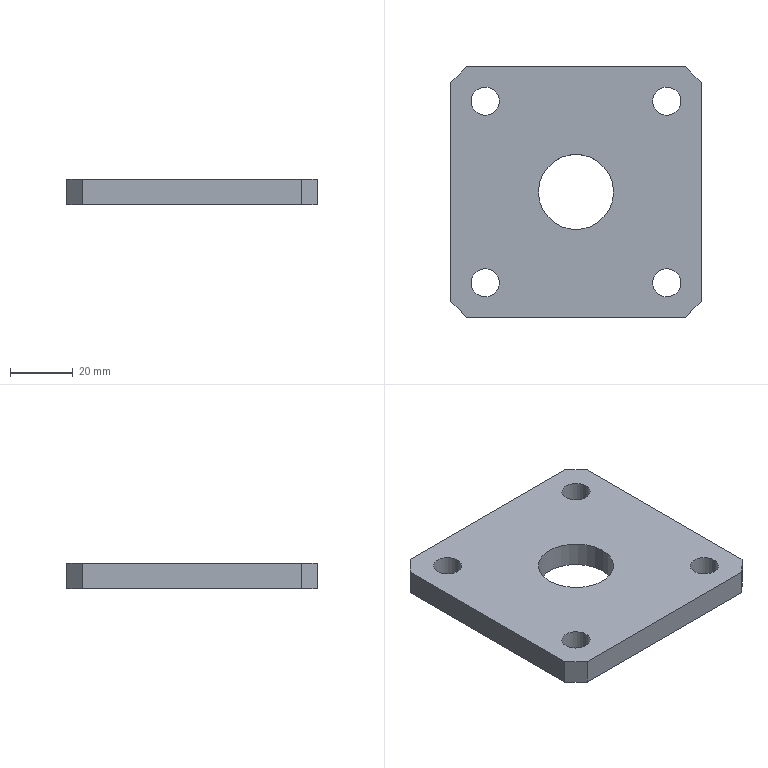Part | SolidWorks | features Chamfer 1, Extrusion 1 | 1 solid | 20 faces | box 80 x 80 x 8 mm | volume 45145 mm3 | cylinder 10 | plane 10 | commonest cylinder face diameters 9 x8 24 x2
STEP:
#1=CARTESIAN_POINT('',(23.386,38.474,8.));
#2=VERTEX_POINT('',#1);
#3=CARTESIAN_POINT('',(32.386,38.474,8.));
#4=VERTEX_POINT('',#3);
#5=CARTESIAN_POINT('',(27.886,38.474,8.));
#6=DIRECTION('',(0.,0.,1.));
#7=DIRECTION('',(1.,0.,0.));
#8=AXIS2_PLACEMENT_3D('',#5,#6,#7);
#9=CIRCLE('',#8,4.5);
#10=EDGE_CURVE('',#2,#4,#9,.T.);
#11=ORIENTED_EDGE('',*,*,#10,.T.);
#12=CARTESIAN_POINT('',(32.386,38.474,0.));
#13=VERTEX_POINT('',#12);
#14=CARTESIAN_POINT('',(32.386,38.474,8.));
#15=DIRECTION('',(0.,0.,-1.));
#16=VECTOR('',#15,1000.);
#17=LINE('',#14,#16);
#18=EDGE_CURVE('',#4,#13,#17,.T.);
#19=ORIENTED_EDGE('',*,*,#18,.T.);
#20=CARTESIAN_POINT('',(23.386,38.474,0.));
#21=VERTEX_POINT('',#20);
#22=CARTESIAN_POINT('',(27.886,38.474,0.));
#23=DIRECTION('',(0.,0.,1.));
#24=DIRECTION('',(1.,0.,0.));
#25=AXIS2_PLACEMENT_3D('',#22,#23,#24);
#26=CIRCLE('',#25,4.5);
#27=EDGE_CURVE('',#21,#13,#26,.T.);
#28=ORIENTED_EDGE('',*,*,#27,.F.);
#29=CARTESIAN_POINT('',(23.386,38.474,8.));
#30=DIRECTION('',(0.,0.,-1.));
#31=VECTOR('',#30,1000.);
#32=LINE('',#29,#31);
#33=EDGE_CURVE('',#2,#21,#32,.T.);
#34=ORIENTED_EDGE('',*,*,#33,.F.);
#35=EDGE_LOOP('',(#11,#19,#28,#34));
#36=FACE_OUTER_BOUND('',#35,.T.);
#37=CARTESIAN_POINT('',(27.886,38.474,8.));
#38=DIRECTION('',(0.,0.,-1.));
#39=DIRECTION('',(-1.,0.,0.));
#40=AXIS2_PLACEMENT_3D('',#37,#38,#39);
#41=CYLINDRICAL_SURFACE('',#40,4.5);
#42=ADVANCED_FACE('',(#36),#41,.F.);
#43=CARTESIAN_POINT('',(23.386,-19.526,8.));
#44=VERTEX_POINT('',#43);
#45=CARTESIAN_POINT('',(32.386,-19.526,8.));
#46=VERTEX_POINT('',#45);
#47=CARTESIAN_POINT('',(27.886,-19.526,8.));
#48=DIRECTION('',(0.,0.,1.));
#49=DIRECTION('',(1.,0.,0.));
#50=AXIS2_PLACEMENT_3D('',#47,#48,#49);
#51=CIRCLE('',#50,4.5);
#52=EDGE_CURVE('',#44,#46,#51,.T.);
#53=ORIENTED_EDGE('',*,*,#52,.T.);
#54=CARTESIAN_POINT('',(32.386,-19.526,0.));
#55=VERTEX_POINT('',#54);
#56=CARTESIAN_POINT('',(32.386,-19.526,8.));
#57=DIRECTION('',(0.,0.,-1.));
#58=VECTOR('',#57,1000.);
#59=LINE('',#56,#58);
#60=EDGE_CURVE('',#46,#55,#59,.T.);
#61=ORIENTED_EDGE('',*,*,#60,.T.);
#62=CARTESIAN_POINT('',(23.386,-19.526,0.));
#63=VERTEX_POINT('',#62);
#64=CARTESIAN_POINT('',(27.886,-19.526,0.));
#65=DIRECTION('',(0.,0.,1.));
#66=DIRECTION('',(1.,0.,0.));
#67=AXIS2_PLACEMENT_3D('',#64,#65,#66);
#68=CIRCLE('',#67,4.5);
#69=EDGE_CURVE('',#63,#55,#68,.T.);
#70=ORIENTED_EDGE('',*,*,#69,.F.);
#71=CARTESIAN_POINT('',(23.386,-19.526,8.));
#72=DIRECTION('',(0.,0.,-1.));
#73=VECTOR('',#72,1000.);
#74=LINE('',#71,#73);
#75=EDGE_CURVE('',#44,#63,#74,.T.);
#76=ORIENTED_EDGE('',*,*,#75,.F.);
#77=EDGE_LOOP('',(#53,#61,#70,#76));
#78=FACE_OUTER_BOUND('',#77,.T.);
#79=CARTESIAN_POINT('',(27.886,-19.526,8.));
#80=DIRECTION('',(0.,0.,-1.));
#81=DIRECTION('',(-1.,0.,0.));
#82=AXIS2_PLACEMENT_3D('',#79,#80,#81);
#83=CYLINDRICAL_SURFACE('',#82,4.5);
#84=ADVANCED_FACE('',(#78),#83,.F.);
#85=CARTESIAN_POINT('',(-34.614,-19.526,8.));
#86=VERTEX_POINT('',#85);
#87=CARTESIAN_POINT('',(-25.614,-19.526,8.));
#88=VERTEX_POINT('',#87);
#89=CARTESIAN_POINT('',(-30.114,-19.526,8.));
#90=DIRECTION('',(0.,0.,1.));
#91=DIRECTION('',(1.,0.,0.));
#92=AXIS2_PLACEMENT_3D('',#89,#90,#91);
#93=CIRCLE('',#92,4.5);
#94=EDGE_CURVE('',#86,#88,#93,.T.);
#95=ORIENTED_EDGE('',*,*,#94,.T.);
#96=CARTESIAN_POINT('',(-25.614,-19.526,0.));
#97=VERTEX_POINT('',#96);
#98=CARTESIAN_POINT('',(-25.614,-19.526,8.));
#99=DIRECTION('',(0.,0.,-1.));
#100=VECTOR('',#99,1000.);
#101=LINE('',#98,#100);
#102=EDGE_CURVE('',#88,#97,#101,.T.);
#103=ORIENTED_EDGE('',*,*,#102,.T.);
#104=CARTESIAN_POINT('',(-34.614,-19.526,0.));
#105=VERTEX_POINT('',#104);
#106=CARTESIAN_POINT('',(-30.114,-19.526,0.));
#107=DIRECTION('',(0.,0.,1.));
#108=DIRECTION('',(1.,0.,0.));
#109=AXIS2_PLACEMENT_3D('',#106,#107,#108);
#110=CIRCLE('',#109,4.5);
#111=EDGE_CURVE('',#105,#97,#110,.T.);
#112=ORIENTED_EDGE('',*,*,#111,.F.);
#113=CARTESIAN_POINT('',(-34.614,-19.526,8.));
#114=DIRECTION('',(0.,0.,-1.));
#115=VECTOR('',#114,1000.);
#116=LINE('',#113,#115);
#117=EDGE_CURVE('',#86,#105,#116,.T.);
#118=ORIENTED_EDGE('',*,*,#117,.F.);
#119=EDGE_LOOP('',(#95,#103,#112,#118));
#120=FACE_OUTER_BOUND('',#119,.T.);
#121=CARTESIAN_POINT('',(-30.114,-19.526,8.));
#122=DIRECTION('',(0.,0.,-1.));
#123=DIRECTION('',(-1.,0.,0.));
#124=AXIS2_PLACEMENT_3D('',#121,#122,#123);
#125=CYLINDRICAL_SURFACE('',#124,4.5);
#126=ADVANCED_FACE('',(#120),#125,.F.);
#127=CARTESIAN_POINT('',(-34.614,38.474,8.));
#128=VERTEX_POINT('',#127);
#129=CARTESIAN_POINT('',(-25.614,38.474,8.));
#130=VERTEX_POINT('',#129);
#131=CARTESIAN_POINT('',(-30.114,38.474,8.));
#132=DIRECTION('',(0.,0.,1.));
#133=DIRECTION('',(1.,0.,0.));
#134=AXIS2_PLACEMENT_3D('',#131,#132,#133);
#135=CIRCLE('',#134,4.5);
#136=EDGE_CURVE('',#128,#130,#135,.T.);
#137=ORIENTED_EDGE('',*,*,#136,.T.);
#138=CARTESIAN_POINT('',(-25.614,38.474,0.));
#139=VERTEX_POINT('',#138);
#140=CARTESIAN_POINT('',(-25.614,38.474,8.));
#141=DIRECTION('',(0.,0.,-1.));
#142=VECTOR('',#141,1000.);
#143=LINE('',#140,#142);
#144=EDGE_CURVE('',#130,#139,#143,.T.);
#145=ORIENTED_EDGE('',*,*,#144,.T.);
#146=CARTESIAN_POINT('',(-34.614,38.474,0.));
#147=VERTEX_POINT('',#146);
#148=CARTESIAN_POINT('',(-30.114,38.474,0.));
#149=DIRECTION('',(0.,0.,1.));
#150=DIRECTION('',(1.,0.,0.));
#151=AXIS2_PLACEMENT_3D('',#148,#149,#150);
#152=CIRCLE('',#151,4.5);
#153=EDGE_CURVE('',#147,#139,#152,.T.);
#154=ORIENTED_EDGE('',*,*,#153,.F.);
#155=CARTESIAN_POINT('',(-34.614,38.474,8.));
#156=DIRECTION('',(0.,0.,-1.));
#157=VECTOR('',#156,1000.);
#158=LINE('',#155,#157);
#159=EDGE_CURVE('',#128,#147,#158,.T.);
#160=ORIENTED_EDGE('',*,*,#159,.F.);
#161=EDGE_LOOP('',(#137,#145,#154,#160));
#162=FACE_OUTER_BOUND('',#161,.T.);
#163=CARTESIAN_POINT('',(-30.114,38.474,8.));
#164=DIRECTION('',(0.,0.,-1.));
#165=DIRECTION('',(-1.,0.,0.));
#166=AXIS2_PLACEMENT_3D('',#163,#164,#165);
#167=CYLINDRICAL_SURFACE('',#166,4.5);
#168=ADVANCED_FACE('',(#162),#167,.F.);
#169=CARTESIAN_POINT('',(-13.114,9.474,8.));
#170=VERTEX_POINT('',#169);
#171=CARTESIAN_POINT('',(10.886,9.474,8.));
#172=VERTEX_POINT('',#171);
#173=CARTESIAN_POINT('',(-1.114,9.474,8.));
#174=DIRECTION('',(0.,0.,1.));
#175=DIRECTION('',(1.,0.,0.));
#176=AXIS2_PLACEMENT_3D('',#173,#174,#175);
#177=CIRCLE('',#176,12.);
#178=EDGE_CURVE('',#170,#172,#177,.T.);
#179=ORIENTED_EDGE('',*,*,#178,.T.);
#180=CARTESIAN_POINT('',(10.886,9.474,0.));
#181=VERTEX_POINT('',#180);
#182=CARTESIAN_POINT('',(10.886,9.474,8.));
#183=DIRECTION('',(0.,0.,-1.));
#184=VECTOR('',#183,1000.);
#185=LINE('',#182,#184);
#186=EDGE_CURVE('',#172,#181,#185,.T.);
#187=ORIENTED_EDGE('',*,*,#186,.T.);
#188=CARTESIAN_POINT('',(-13.114,9.474,0.));
#189=VERTEX_POINT('',#188);
#190=CARTESIAN_POINT('',(-1.114,9.474,0.));
#191=DIRECTION('',(0.,0.,1.));
#192=DIRECTION('',(1.,0.,0.));
#193=AXIS2_PLACEMENT_3D('',#190,#191,#192);
#194=CIRCLE('',#193,12.);
#195=EDGE_CURVE('',#189,#181,#194,.T.);
#196=ORIENTED_EDGE('',*,*,#195,.F.);
#197=CARTESIAN_POINT('',(-13.114,9.474,8.));
#198=DIRECTION('',(0.,0.,-1.));
#199=VECTOR('',#198,1000.);
#200=LINE('',#197,#199);
#201=EDGE_CURVE('',#170,#189,#200,.T.);
#202=ORIENTED_EDGE('',*,*,#201,.F.);
#203=EDGE_LOOP('',(#179,#187,#196,#202));
#204=FACE_OUTER_BOUND('',#203,.T.);
#205=CARTESIAN_POINT('',(-1.114,9.474,8.));
#206=DIRECTION('',(0.,0.,-1.));
#207=DIRECTION('',(-1.,0.,0.));
#208=AXIS2_PLACEMENT_3D('',#205,#206,#207);
#209=CYLINDRICAL_SURFACE('',#208,12.);
#210=ADVANCED_FACE('',(#204),#209,.F.);
#211=ORIENTED_EDGE('',*,*,#52,.F.);
#212=CARTESIAN_POINT('',(27.886,-19.526,8.));
#213=DIRECTION('',(0.,0.,1.));
#214=DIRECTION('',(1.,0.,0.));
#215=AXIS2_PLACEMENT_3D('',#212,#213,#214);
#216=CIRCLE('',#215,4.5);
#217=EDGE_CURVE('',#46,#44,#216,.T.);
#218=ORIENTED_EDGE('',*,*,#217,.F.);
#219=EDGE_LOOP('',(#211,#218));
#220=FACE_BOUND('',#219,.T.);
#221=ORIENTED_EDGE('',*,*,#136,.F.);
#222=CARTESIAN_POINT('',(-30.114,38.474,8.));
#223=DIRECTION('',(0.,0.,1.));
#224=DIRECTION('',(1.,0.,0.));
#225=AXIS2_PLACEMENT_3D('',#222,#223,#224);
#226=CIRCLE('',#225,4.5);
#227=EDGE_CURVE('',#130,#128,#226,.T.);
#228=ORIENTED_EDGE('',*,*,#227,.F.);
#229=EDGE_LOOP('',(#221,#228));
#230=FACE_BOUND('',#229,.T.);
#231=CARTESIAN_POINT('',(-36.114,-30.526,8.));
#232=VERTEX_POINT('',#231);
#233=CARTESIAN_POINT('',(33.886,-30.526,8.));
#234=VERTEX_POINT('',#233);
#235=CARTESIAN_POINT('',(-41.114,-30.526,8.));
#236=DIRECTION('',(1.,0.,0.));
#237=VECTOR('',#236,1000.);
#238=LINE('',#235,#237);
#239=EDGE_CURVE('',#232,#234,#238,.T.);
#240=ORIENTED_EDGE('',*,*,#239,.T.);
#241=CARTESIAN_POINT('',(38.886,-25.526,8.));
#242=VERTEX_POINT('',#241);
#243=CARTESIAN_POINT('',(32.206,-32.206,8.));
#244=DIRECTION('',(0.7071,0.7071,0.));
#245=VECTOR('',#244,1000.);
#246=LINE('',#243,#245);
#247=EDGE_CURVE('',#234,#242,#246,.T.);
#248=ORIENTED_EDGE('',*,*,#247,.T.);
#249=CARTESIAN_POINT('',(38.886,44.474,8.));
#250=VERTEX_POINT('',#249);
#251=CARTESIAN_POINT('',(38.886,49.474,8.));
#252=DIRECTION('',(0.,1.,0.));
#253=VECTOR('',#252,1000.);
#254=LINE('',#251,#253);
#255=EDGE_CURVE('',#242,#250,#254,.T.);
#256=ORIENTED_EDGE('',*,*,#255,.T.);
#257=CARTESIAN_POINT('',(33.886,49.474,8.));
#258=VERTEX_POINT('',#257);
#259=CARTESIAN_POINT('',(41.68,41.68,8.));
#260=DIRECTION('',(-0.7071,0.7071,0.));
#261=VECTOR('',#260,1000.);
#262=LINE('',#259,#261);
#263=EDGE_CURVE('',#250,#258,#262,.T.);
#264=ORIENTED_EDGE('',*,*,#263,.T.);
#265=CARTESIAN_POINT('',(-36.114,49.474,8.));
#266=VERTEX_POINT('',#265);
#267=CARTESIAN_POINT('',(-41.114,49.474,8.));
#268=DIRECTION('',(-1.,0.,0.));
#269=VECTOR('',#268,1000.);
#270=LINE('',#267,#269);
#271=EDGE_CURVE('',#258,#266,#270,.T.);
#272=ORIENTED_EDGE('',*,*,#271,.T.);
#273=CARTESIAN_POINT('',(-41.114,44.474,8.));
#274=VERTEX_POINT('',#273);
#275=CARTESIAN_POINT('',(-42.794,42.794,8.));
#276=DIRECTION('',(-0.7071,-0.7071,0.));
#277=VECTOR('',#276,1000.);
#278=LINE('',#275,#277);
#279=EDGE_CURVE('',#266,#274,#278,.T.);
#280=ORIENTED_EDGE('',*,*,#279,.T.);
#281=CARTESIAN_POINT('',(-41.114,-25.526,8.));
#282=VERTEX_POINT('',#281);
#283=CARTESIAN_POINT('',(-41.114,49.474,8.));
#284=DIRECTION('',(0.,-1.,0.));
#285=VECTOR('',#284,1000.);
#286=LINE('',#283,#285);
#287=EDGE_CURVE('',#274,#282,#286,.T.);
#288=ORIENTED_EDGE('',*,*,#287,.T.);
#289=CARTESIAN_POINT('',(-33.32,-33.32,8.));
#290=DIRECTION('',(0.7071,-0.7071,0.));
#291=VECTOR('',#290,1000.);
#292=LINE('',#289,#291);
#293=EDGE_CURVE('',#282,#232,#292,.T.);
#294=ORIENTED_EDGE('',*,*,#293,.T.);
#295=EDGE_LOOP('',(#240,#248,#256,#264,#272,#280,#288,#294));
#296=FACE_OUTER_BOUND('',#295,.T.);
#297=ORIENTED_EDGE('',*,*,#178,.F.);
#298=CARTESIAN_POINT('',(-1.114,9.474,8.));
#299=DIRECTION('',(0.,0.,1.));
#300=DIRECTION('',(1.,0.,0.));
#301=AXIS2_PLACEMENT_3D('',#298,#299,#300);
#302=CIRCLE('',#301,12.);
#303=EDGE_CURVE('',#172,#170,#302,.T.);
#304=ORIENTED_EDGE('',*,*,#303,.F.);
#305=EDGE_LOOP('',(#297,#304));
#306=FACE_BOUND('',#305,.T.);
#307=ORIENTED_EDGE('',*,*,#94,.F.);
#308=CARTESIAN_POINT('',(-30.114,-19.526,8.));
#309=DIRECTION('',(0.,0.,1.));
#310=DIRECTION('',(1.,0.,0.));
#311=AXIS2_PLACEMENT_3D('',#308,#309,#310);
#312=CIRCLE('',#311,4.5);
#313=EDGE_CURVE('',#88,#86,#312,.T.);
#314=ORIENTED_EDGE('',*,*,#313,.F.);
#315=EDGE_LOOP('',(#307,#314));
#316=FACE_BOUND('',#315,.T.);
#317=ORIENTED_EDGE('',*,*,#10,.F.);
#318=CARTESIAN_POINT('',(27.886,38.474,8.));
#319=DIRECTION('',(0.,0.,1.));
#320=DIRECTION('',(1.,0.,0.));
#321=AXIS2_PLACEMENT_3D('',#318,#319,#320);
#322=CIRCLE('',#321,4.5);
#323=EDGE_CURVE('',#4,#2,#322,.T.);
#324=ORIENTED_EDGE('',*,*,#323,.F.);
#325=EDGE_LOOP('',(#317,#324));
#326=FACE_BOUND('',#325,.T.);
#327=CARTESIAN_POINT('',(0.,0.,8.));
#328=DIRECTION('',(0.,0.,1.));
#329=DIRECTION('',(1.,0.,0.));
#330=AXIS2_PLACEMENT_3D('',#327,#328,#329);
#331=PLANE('',#330);
#332=ADVANCED_FACE('',(#220,#230,#296,#306,#316,#326),#331,.T.);
#333=CARTESIAN_POINT('',(38.886,-25.526,0.));
#334=VERTEX_POINT('',#333);
#335=CARTESIAN_POINT('',(38.886,44.474,0.));
#336=VERTEX_POINT('',#335);
#337=CARTESIAN_POINT('',(38.886,49.474,0.));
#338=DIRECTION('',(0.,1.,0.));
#339=VECTOR('',#338,1000.);
#340=LINE('',#337,#339);
#341=EDGE_CURVE('',#334,#336,#340,.T.);
#342=ORIENTED_EDGE('',*,*,#341,.F.);
#343=CARTESIAN_POINT('',(33.886,-30.526,0.));
#344=VERTEX_POINT('',#343);
#345=CARTESIAN_POINT('',(38.886,-25.526,0.));
#346=DIRECTION('',(-0.7071,-0.7071,0.));
#347=VECTOR('',#346,1000.);
#348=LINE('',#345,#347);
#349=EDGE_CURVE('',#334,#344,#348,.T.);
#350=ORIENTED_EDGE('',*,*,#349,.T.);
#351=CARTESIAN_POINT('',(-36.114,-30.526,0.));
#352=VERTEX_POINT('',#351);
#353=CARTESIAN_POINT('',(-41.114,-30.526,0.));
#354=DIRECTION('',(1.,0.,0.));
#355=VECTOR('',#354,1000.);
#356=LINE('',#353,#355);
#357=EDGE_CURVE('',#352,#344,#356,.T.);
#358=ORIENTED_EDGE('',*,*,#357,.F.);
#359=CARTESIAN_POINT('',(-41.114,-25.526,0.));
#360=VERTEX_POINT('',#359);
#361=CARTESIAN_POINT('',(-36.114,-30.526,0.));
#362=DIRECTION('',(-0.7071,0.7071,0.));
#363=VECTOR('',#362,1000.);
#364=LINE('',#361,#363);
#365=EDGE_CURVE('',#352,#360,#364,.T.);
#366=ORIENTED_EDGE('',*,*,#365,.T.);
#367=CARTESIAN_POINT('',(-41.114,44.474,0.));
#368=VERTEX_POINT('',#367);
#369=CARTESIAN_POINT('',(-41.114,49.474,0.));
#370=DIRECTION('',(0.,-1.,0.));
#371=VECTOR('',#370,1000.);
#372=LINE('',#369,#371);
#373=EDGE_CURVE('',#368,#360,#372,.T.);
#374=ORIENTED_EDGE('',*,*,#373,.F.);
#375=CARTESIAN_POINT('',(-36.114,49.474,0.));
#376=VERTEX_POINT('',#375);
#377=CARTESIAN_POINT('',(-41.114,44.474,0.));
#378=DIRECTION('',(0.7071,0.7071,0.));
#379=VECTOR('',#378,1000.);
#380=LINE('',#377,#379);
#381=EDGE_CURVE('',#368,#376,#380,.T.);
#382=ORIENTED_EDGE('',*,*,#381,.T.);
#383=CARTESIAN_POINT('',(33.886,49.474,0.));
#384=VERTEX_POINT('',#383);
#385=CARTESIAN_POINT('',(-41.114,49.474,0.));
#386=DIRECTION('',(-1.,0.,0.));
#387=VECTOR('',#386,1000.);
#388=LINE('',#385,#387);
#389=EDGE_CURVE('',#384,#376,#388,.T.);
#390=ORIENTED_EDGE('',*,*,#389,.F.);
#391=CARTESIAN_POINT('',(33.886,49.474,0.));
#392=DIRECTION('',(0.7071,-0.7071,0.));
#393=VECTOR('',#392,1000.);
#394=LINE('',#391,#393);
#395=EDGE_CURVE('',#384,#336,#394,.T.);
#396=ORIENTED_EDGE('',*,*,#395,.T.);
#397=EDGE_LOOP('',(#342,#350,#358,#366,#374,#382,#390,#396));
#398=FACE_OUTER_BOUND('',#397,.T.);
#399=ORIENTED_EDGE('',*,*,#195,.T.);
#400=CARTESIAN_POINT('',(-1.114,9.474,0.));
#401=DIRECTION('',(0.,0.,1.));
#402=DIRECTION('',(1.,0.,0.));
#403=AXIS2_PLACEMENT_3D('',#400,#401,#402);
#404=CIRCLE('',#403,12.);
#405=EDGE_CURVE('',#181,#189,#404,.T.);
#406=ORIENTED_EDGE('',*,*,#405,.T.);
#407=EDGE_LOOP('',(#399,#406));
#408=FACE_BOUND('',#407,.T.);
#409=ORIENTED_EDGE('',*,*,#153,.T.);
#410=CARTESIAN_POINT('',(-30.114,38.474,0.));
#411=DIRECTION('',(0.,0.,1.));
#412=DIRECTION('',(1.,0.,0.));
#413=AXIS2_PLACEMENT_3D('',#410,#411,#412);
#414=CIRCLE('',#413,4.5);
#415=EDGE_CURVE('',#139,#147,#414,.T.);
#416=ORIENTED_EDGE('',*,*,#415,.T.);
#417=EDGE_LOOP('',(#409,#416));
#418=FACE_BOUND('',#417,.T.);
#419=ORIENTED_EDGE('',*,*,#111,.T.);
#420=CARTESIAN_POINT('',(-30.114,-19.526,0.));
#421=DIRECTION('',(0.,0.,1.));
#422=DIRECTION('',(1.,0.,0.));
#423=AXIS2_PLACEMENT_3D('',#420,#421,#422);
#424=CIRCLE('',#423,4.5);
#425=EDGE_CURVE('',#97,#105,#424,.T.);
#426=ORIENTED_EDGE('',*,*,#425,.T.);
#427=EDGE_LOOP('',(#419,#426));
#428=FACE_BOUND('',#427,.T.);
#429=ORIENTED_EDGE('',*,*,#69,.T.);
#430=CARTESIAN_POINT('',(27.886,-19.526,0.));
#431=DIRECTION('',(0.,0.,1.));
#432=DIRECTION('',(1.,0.,0.));
#433=AXIS2_PLACEMENT_3D('',#430,#431,#432);
#434=CIRCLE('',#433,4.5);
#435=EDGE_CURVE('',#55,#63,#434,.T.);
#436=ORIENTED_EDGE('',*,*,#435,.T.);
#437=EDGE_LOOP('',(#429,#436));
#438=FACE_BOUND('',#437,.T.);
#439=ORIENTED_EDGE('',*,*,#27,.T.);
#440=CARTESIAN_POINT('',(27.886,38.474,0.));
#441=DIRECTION('',(0.,0.,1.));
#442=DIRECTION('',(1.,0.,0.));
#443=AXIS2_PLACEMENT_3D('',#440,#441,#442);
#444=CIRCLE('',#443,4.5);
#445=EDGE_CURVE('',#13,#21,#444,.T.);
#446=ORIENTED_EDGE('',*,*,#445,.T.);
#447=EDGE_LOOP('',(#439,#446));
#448=FACE_BOUND('',#447,.T.);
#449=CARTESIAN_POINT('',(0.,0.,0.));
#450=DIRECTION('',(0.,0.,1.));
#451=DIRECTION('',(1.,0.,0.));
#452=AXIS2_PLACEMENT_3D('',#449,#450,#451);
#453=PLANE('',#452);
#454=ADVANCED_FACE('',(#398,#408,#418,#428,#438,#448),#453,.F.);
#455=ORIENTED_EDGE('',*,*,#373,.T.);
#456=CARTESIAN_POINT('',(-41.114,-25.526,8.));
#457=DIRECTION('',(0.,0.,1.));
#458=VECTOR('',#457,1000.);
#459=LINE('',#456,#458);
#460=EDGE_CURVE('',#360,#282,#459,.T.);
#461=ORIENTED_EDGE('',*,*,#460,.T.);
#462=ORIENTED_EDGE('',*,*,#287,.F.);
#463=CARTESIAN_POINT('',(-41.114,44.474,8.));
#464=DIRECTION('',(0.,0.,-1.));
#465=VECTOR('',#464,1000.);
#466=LINE('',#463,#465);
#467=EDGE_CURVE('',#274,#368,#466,.T.);
#468=ORIENTED_EDGE('',*,*,#467,.T.);
#469=EDGE_LOOP('',(#455,#461,#462,#468));
#470=FACE_OUTER_BOUND('',#469,.T.);
#471=CARTESIAN_POINT('',(-41.114,49.474,8.));
#472=DIRECTION('',(1.,0.,0.));
#473=DIRECTION('',(0.,1.,0.));
#474=AXIS2_PLACEMENT_3D('',#471,#472,#473);
#475=PLANE('',#474);
#476=ADVANCED_FACE('',(#470),#475,.F.);
#477=ORIENTED_EDGE('',*,*,#357,.T.);
#478=CARTESIAN_POINT('',(33.886,-30.526,8.));
#479=DIRECTION('',(0.,0.,1.));
#480=VECTOR('',#479,1000.);
#481=LINE('',#478,#480);
#482=EDGE_CURVE('',#344,#234,#481,.T.);
#483=ORIENTED_EDGE('',*,*,#482,.T.);
#484=ORIENTED_EDGE('',*,*,#239,.F.);
#485=CARTESIAN_POINT('',(-36.114,-30.526,8.));
#486=DIRECTION('',(0.,0.,-1.));
#487=VECTOR('',#486,1000.);
#488=LINE('',#485,#487);
#489=EDGE_CURVE('',#232,#352,#488,.T.);
#490=ORIENTED_EDGE('',*,*,#489,.T.);
#491=EDGE_LOOP('',(#477,#483,#484,#490));
#492=FACE_OUTER_BOUND('',#491,.T.);
#493=CARTESIAN_POINT('',(-41.114,-30.526,8.));
#494=DIRECTION('',(0.,1.,0.));
#495=DIRECTION('',(0.,0.,1.));
#496=AXIS2_PLACEMENT_3D('',#493,#494,#495);
#497=PLANE('',#496);
#498=ADVANCED_FACE('',(#492),#497,.F.);
#499=ORIENTED_EDGE('',*,*,#255,.F.);
#500=CARTESIAN_POINT('',(38.886,-25.526,8.));
#501=DIRECTION('',(0.,0.,-1.));
#502=VECTOR('',#501,1000.);
#503=LINE('',#500,#502);
#504=EDGE_CURVE('',#242,#334,#503,.T.);
#505=ORIENTED_EDGE('',*,*,#504,.T.);
#506=ORIENTED_EDGE('',*,*,#341,.T.);
#507=CARTESIAN_POINT('',(38.886,44.474,8.));
#508=DIRECTION('',(0.,0.,1.));
#509=VECTOR('',#508,1000.);
#510=LINE('',#507,#509);
#511=EDGE_CURVE('',#336,#250,#510,.T.);
#512=ORIENTED_EDGE('',*,*,#511,.T.);
#513=EDGE_LOOP('',(#499,#505,#506,#512));
#514=FACE_OUTER_BOUND('',#513,.T.);
#515=CARTESIAN_POINT('',(38.886,49.474,8.));
#516=DIRECTION('',(-1.,0.,0.));
#517=DIRECTION('',(0.,-1.,0.));
#518=AXIS2_PLACEMENT_3D('',#515,#516,#517);
#519=PLANE('',#518);
#520=ADVANCED_FACE('',(#514),#519,.F.);
#521=ORIENTED_EDGE('',*,*,#271,.F.);
#522=CARTESIAN_POINT('',(33.886,49.474,8.));
#523=DIRECTION('',(0.,0.,-1.));
#524=VECTOR('',#523,1000.);
#525=LINE('',#522,#524);
#526=EDGE_CURVE('',#258,#384,#525,.T.);
#527=ORIENTED_EDGE('',*,*,#526,.T.);
#528=ORIENTED_EDGE('',*,*,#389,.T.);
#529=CARTESIAN_POINT('',(-36.114,49.474,8.));
#530=DIRECTION('',(0.,0.,1.));
#531=VECTOR('',#530,1000.);
#532=LINE('',#529,#531);
#533=EDGE_CURVE('',#376,#266,#532,.T.);
#534=ORIENTED_EDGE('',*,*,#533,.T.);
#535=EDGE_LOOP('',(#521,#527,#528,#534));
#536=FACE_OUTER_BOUND('',#535,.T.);
#537=CARTESIAN_POINT('',(-41.114,49.474,8.));
#538=DIRECTION('',(0.,-1.,0.));
#539=DIRECTION('',(0.,0.,-1.));
#540=AXIS2_PLACEMENT_3D('',#537,#538,#539);
#541=PLANE('',#540);
#542=ADVANCED_FACE('',(#536),#541,.F.);
#543=ORIENTED_EDGE('',*,*,#186,.F.);
#544=ORIENTED_EDGE('',*,*,#303,.T.);
#545=ORIENTED_EDGE('',*,*,#201,.T.);
#546=ORIENTED_EDGE('',*,*,#405,.F.);
#547=EDGE_LOOP('',(#543,#544,#545,#546));
#548=FACE_OUTER_BOUND('',#547,.T.);
#549=CARTESIAN_POINT('',(-1.114,9.474,8.));
#550=DIRECTION('',(0.,0.,-1.));
#551=DIRECTION('',(-1.,0.,0.));
#552=AXIS2_PLACEMENT_3D('',#549,#550,#551);
#553=CYLINDRICAL_SURFACE('',#552,12.);
#554=ADVANCED_FACE('',(#548),#553,.F.);
#555=ORIENTED_EDGE('',*,*,#144,.F.);
#556=ORIENTED_EDGE('',*,*,#227,.T.);
#557=ORIENTED_EDGE('',*,*,#159,.T.);
#558=ORIENTED_EDGE('',*,*,#415,.F.);
#559=EDGE_LOOP('',(#555,#556,#557,#558));
#560=FACE_OUTER_BOUND('',#559,.T.);
#561=CARTESIAN_POINT('',(-30.114,38.474,8.));
#562=DIRECTION('',(0.,0.,-1.));
#563=DIRECTION('',(-1.,0.,0.));
#564=AXIS2_PLACEMENT_3D('',#561,#562,#563);
#565=CYLINDRICAL_SURFACE('',#564,4.5);
#566=ADVANCED_FACE('',(#560),#565,.F.);
#567=ORIENTED_EDGE('',*,*,#102,.F.);
#568=ORIENTED_EDGE('',*,*,#313,.T.);
#569=ORIENTED_EDGE('',*,*,#117,.T.);
#570=ORIENTED_EDGE('',*,*,#425,.F.);
#571=EDGE_LOOP('',(#567,#568,#569,#570));
#572=FACE_OUTER_BOUND('',#571,.T.);
#573=CARTESIAN_POINT('',(-30.114,-19.526,8.));
#574=DIRECTION('',(0.,0.,-1.));
#575=DIRECTION('',(-1.,0.,0.));
#576=AXIS2_PLACEMENT_3D('',#573,#574,#575);
#577=CYLINDRICAL_SURFACE('',#576,4.5);
#578=ADVANCED_FACE('',(#572),#577,.F.);
#579=ORIENTED_EDGE('',*,*,#60,.F.);
#580=ORIENTED_EDGE('',*,*,#217,.T.);
#581=ORIENTED_EDGE('',*,*,#75,.T.);
#582=ORIENTED_EDGE('',*,*,#435,.F.);
#583=EDGE_LOOP('',(#579,#580,#581,#582));
#584=FACE_OUTER_BOUND('',#583,.T.);
#585=CARTESIAN_POINT('',(27.886,-19.526,8.));
#586=DIRECTION('',(0.,0.,-1.));
#587=DIRECTION('',(-1.,0.,0.));
#588=AXIS2_PLACEMENT_3D('',#585,#586,#587);
#589=CYLINDRICAL_SURFACE('',#588,4.5);
#590=ADVANCED_FACE('',(#584),#589,.F.);
#591=ORIENTED_EDGE('',*,*,#18,.F.);
#592=ORIENTED_EDGE('',*,*,#323,.T.);
#593=ORIENTED_EDGE('',*,*,#33,.T.);
#594=ORIENTED_EDGE('',*,*,#445,.F.);
#595=EDGE_LOOP('',(#591,#592,#593,#594));
#596=FACE_OUTER_BOUND('',#595,.T.);
#597=CARTESIAN_POINT('',(27.886,38.474,8.));
#598=DIRECTION('',(0.,0.,-1.));
#599=DIRECTION('',(-1.,0.,0.));
#600=AXIS2_PLACEMENT_3D('',#597,#598,#599);
#601=CYLINDRICAL_SURFACE('',#600,4.5);
#602=ADVANCED_FACE('',(#596),#601,.F.);
#603=ORIENTED_EDGE('',*,*,#247,.F.);
#604=ORIENTED_EDGE('',*,*,#482,.F.);
#605=ORIENTED_EDGE('',*,*,#349,.F.);
#606=ORIENTED_EDGE('',*,*,#504,.F.);
#607=EDGE_LOOP('',(#603,#604,#605,#606));
#608=FACE_OUTER_BOUND('',#607,.T.);
#609=CARTESIAN_POINT('',(38.886,-25.526,8.));
#610=DIRECTION('',(-0.7071,0.7071,0.));
#611=DIRECTION('',(0.,0.,-1.));
#612=AXIS2_PLACEMENT_3D('',#609,#610,#611);
#613=PLANE('',#612);
#614=ADVANCED_FACE('',(#608),#613,.F.);
#615=ORIENTED_EDGE('',*,*,#263,.F.);
#616=ORIENTED_EDGE('',*,*,#511,.F.);
#617=ORIENTED_EDGE('',*,*,#395,.F.);
#618=ORIENTED_EDGE('',*,*,#526,.F.);
#619=EDGE_LOOP('',(#615,#616,#617,#618));
#620=FACE_OUTER_BOUND('',#619,.T.);
#621=CARTESIAN_POINT('',(33.886,49.474,8.));
#622=DIRECTION('',(-0.7071,-0.7071,0.));
#623=DIRECTION('',(0.,0.,-1.));
#624=AXIS2_PLACEMENT_3D('',#621,#622,#623);
#625=PLANE('',#624);
#626=ADVANCED_FACE('',(#620),#625,.F.);
#627=ORIENTED_EDGE('',*,*,#293,.F.);
#628=ORIENTED_EDGE('',*,*,#460,.F.);
#629=ORIENTED_EDGE('',*,*,#365,.F.);
#630=ORIENTED_EDGE('',*,*,#489,.F.);
#631=EDGE_LOOP('',(#627,#628,#629,#630));
#632=FACE_OUTER_BOUND('',#631,.T.);
#633=CARTESIAN_POINT('',(-36.114,-30.526,8.));
#634=DIRECTION('',(0.7071,0.7071,0.));
#635=DIRECTION('',(0.,0.,-1.));
#636=AXIS2_PLACEMENT_3D('',#633,#634,#635);
#637=PLANE('',#636);
#638=ADVANCED_FACE('',(#632),#637,.F.);
#639=ORIENTED_EDGE('',*,*,#279,.F.);
#640=ORIENTED_EDGE('',*,*,#533,.F.);
#641=ORIENTED_EDGE('',*,*,#381,.F.);
#642=ORIENTED_EDGE('',*,*,#467,.F.);
#643=EDGE_LOOP('',(#639,#640,#641,#642));
#644=FACE_OUTER_BOUND('',#643,.T.);
#645=CARTESIAN_POINT('',(-41.114,44.474,8.));
#646=DIRECTION('',(0.7071,-0.7071,0.));
#647=DIRECTION('',(0.,0.,-1.));
#648=AXIS2_PLACEMENT_3D('',#645,#646,#647);
#649=PLANE('',#648);
#650=ADVANCED_FACE('',(#644),#649,.F.);
#651=CLOSED_SHELL('',(#42,#84,#126,#168,#210,#332,#454,#476,#498,#520,#542,#554,#566,#578,#590,#602,#614,#626,#638,#650));
#652=MANIFOLD_SOLID_BREP('',#651);
#653=CARTESIAN_POINT('',(0.,0.,0.));
#654=DIRECTION('',(0.,0.,1.));
#655=DIRECTION('',(1.,0.,0.));
#656=AXIS2_PLACEMENT_3D('',#653,#654,#655);
#657=(LENGTH_UNIT()NAMED_UNIT(*)SI_UNIT(.MILLI.,.METRE.));
#658=UNCERTAINTY_MEASURE_WITH_UNIT(LENGTH_MEASURE(0.00001),#657,'','');
#659=(NAMED_UNIT(*)PLANE_ANGLE_UNIT()SI_UNIT($,.RADIAN.));
#660=(NAMED_UNIT(*)SI_UNIT($,.STERADIAN.)SOLID_ANGLE_UNIT());
#661=(GEOMETRIC_REPRESENTATION_CONTEXT(3)GLOBAL_UNCERTAINTY_ASSIGNED_CONTEXT((#658))GLOBAL_UNIT_ASSIGNED_CONTEXT((#657,#659,#660))REPRESENTATION_CONTEXT('',''));
#662=ADVANCED_BREP_SHAPE_REPRESENTATION('',(#652,#656),#661);